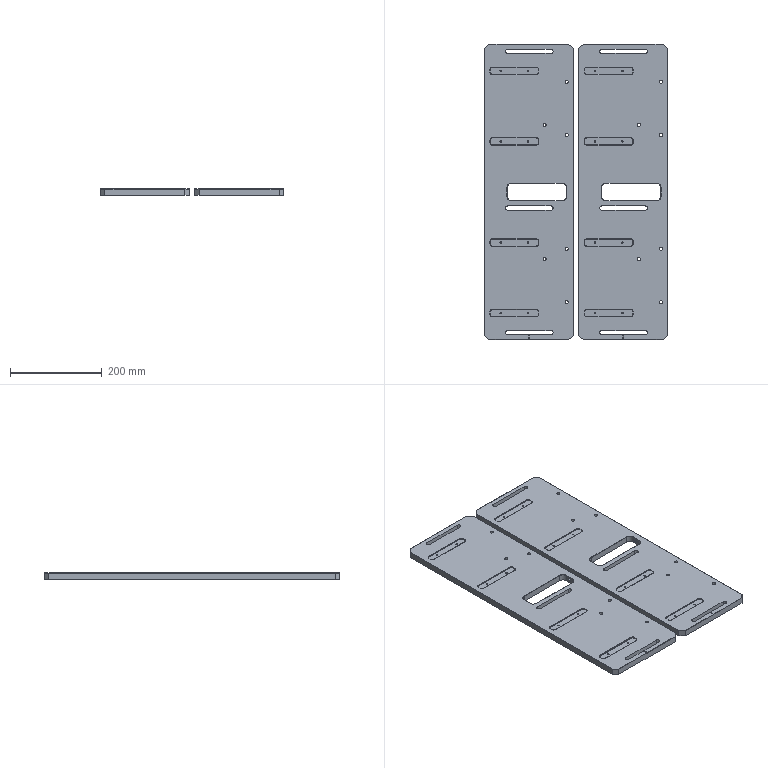CAM job | NX | 3-axis milling, drilling | part box 401 x 645 x 14 mm | stock box 406 x 650 x 14 mm
Tools:
number,name,description,diameter,corner_radius,flute_length,length,flutes
6,D6,平底铣刀-粗,6.0,0.0,25.0,75.0,2
9,D10,平底铣刀-粗,10.0,0.0,35.0,75.0,2
7,D6-J,平底铣刀-精,6.0,0.0,25.0,75.0,2
2,D6倒角刀,倒角刀,6.0,0.0,3.0,25.0,2
21,M4X0.7,丝锥,3.3,0.0,35.0,50.0,2
19,M8X1.25,丝锥,6.8,0.0,35.0,50.0,2
13,ZT3.3,钻头,3.3,0.0,35.0,50.0,2
16,ZT6.8,钻头,6.8,0.0,35.0,50.0,2
Operations:
program,operation,operation_type,tool,method,geometry_group,spindle_rpm,surface_speed,feed_per_tooth,feed_cut,feed_plunge,cut_length_mm,path_length_mm,cut_time_min,machine_time_min
B,打点-深0.8,Operation,D6倒角刀,NONE,W-B,8000.0,150.796,0.0312,500.0,90.0,25.2,1180.181,0.0504,0.1659
B,通孔-M4螺纹底孔,Operation,ZT3.3,NONE,W-B,3000.0,30.159,0.05,300.0,90.0,152.0,1120.042,0.5067,0.6035
B,通孔-M8螺纹底孔,Operation,ZT6.8,NONE,W-B,1800.0,38.453,0.0972,350.0,90.0,144.258,900.607,0.4122,0.4878
B,钻倒角_2,Operation,D6倒角刀,METHOD,W-B,8000.0,150.796,0.0312,500.0,0.0,41.2,912.779,0.0824,0.1696
B,铣倒角_2,PlanarMilling,D6倒角刀,METHOD,W-B,8000.0,150.796,0.0375,600.0,100.0,146.407,952.42,0.244,0.3246
B,C0.3封闭铣廓倒角6X45L_COPY_1,PlanarMilling,D6倒角刀,爬面_倒角-切深0-步距G,W-B,7000.0,131.0,0.1071,1500.0,100.0,2682.246,4133.944,1.788,1.933
B,通孔-攻牙M4,Operation,M4X0.7,METHOD,W-B,600.0,6.22,0.0006,0.7,90.0,8.0,832.042,11.429,11.511
B,通孔-攻牙M8,Operation,M8X1.25,METHOD,W-B,500.0,10.681,0.0013,1.25,90.0,114.0,840.092,91.2,91.273
A,台阶粗_2,CavityMilling,D10,METHOD,W-A,6000.0,188.0,0.25,3500.0,100.0,12611.021,15267.001,3.693,3.958
A,框开粗_1,VolumeBased25DMillingOperation,D10,METHOD,W-A,6000.0,188.0,0.25,4000.0,80.0,17210.28,17519.78,4.303,4.333
A,通腰槽粗_1,VolumeBased25DMillingOperation,D6,METHOD,W-A,6000.0,113.0,0.2083,2500.0,100.0,35792.469,37342.57,14.317,14.472
A,外形粗_2,VolumeBased25DMillingOperation,D10,METHOD,W-A,6000.0,188.0,0.25,4000.0,80.0,94565.32,95081.52,23.641,23.693
A,底精_1,VolumeBased25DMillingOperation,D6-J,METHOD,W-A,6000.0,113.0,0.2083,1200.0,100.0,3578.096,5284.582,2.982,3.152
A,底侧精_3,VolumeBased25DMillingOperation,D6-J,METHOD,W-A,6000.0,113.0,0.2083,1200.0,100.0,1758.464,3353.459,1.465,1.625
A,框半精_1,VolumeBased25DMillingOperation,D6-J,METHOD,W-A,6000.0,113.0,0.0833,1000.0,100.0,1220.431,1561.861,1.22,1.255
A,框精_1,VolumeBased25DMillingOperation,D6-J,METHOD,W-A,6000.0,113.0,0.0833,1000.0,100.0,609.816,951.516,0.6098,0.644
A,腰槽精_1,VolumeBased25DMillingOperation,D6-J,METHOD,W-A,6000.0,113.0,0.0667,800.0,100.0,3629.756,5398.958,4.537,4.714
A,打点,Operation,D6倒角刀,METHOD,W-A,3000.0,56.549,0.0333,200.0,0.0,48.0,1547.83,0.24,0.39
A,仅选体,SurfaceContour,D6倒角刀,METHOD,W-A,6000.0,113.0,0.125,1200.0,100.0,1312.8,3405.337,1.094,1.303
A,钻倒角_1,Operation,D6倒角刀,METHOD,W-A,5000.0,94.248,0.015,150.0,0.0,82.4,1847.602,0.5493,0.7259
A,铣倒角_1,PlanarMilling,D6倒角刀,METHOD,W-A,6000.0,113.097,0.05,600.0,100.0,286.984,2054.873,0.4783,0.6551
A,平面去毛刺6X45L_COPY,SurfaceContour,D6倒角刀,爬面_倒角-切深0-步距G,W-A,6500.0,122.519,0.1154,1500.0,100.0,7452.823,13343.935,4.968,5.558
A,C0.3封闭铣廓倒角6X45L_COPY,PlanarMilling,D6倒角刀,爬面_倒角-切深0-步距G,W-A,7000.0,131.0,0.0214,300.0,100.0,59.0,340.452,0.1967,0.2248
A,外形半精_2,VolumeBased25DMillingOperation,D6-J,METHOD,W-A,6000.0,113.0,0.0833,1000.0,100.0,6721.337,7711.055,6.721,6.82
A,外形精_2,VolumeBased25DMillingOperation,D6-J,METHOD,W-A,6000.0,113.0,0.0833,1000.0,100.0,3360.269,4240.026,3.36,3.448